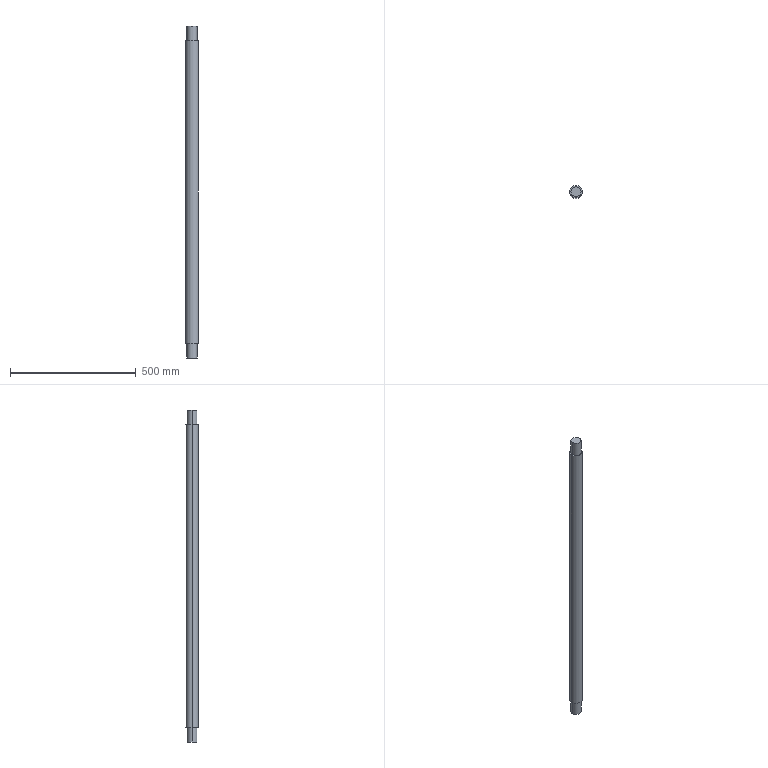Part | STEP file | Double sprocket shaft 1XG | 1 solid | 22 faces | box 50 x 50 x 1320 mm | volume 2495026 mm3 | cylinder 12 | plane 10 | commonest cylinder face diameters 12 x6 40 x4 50 x2